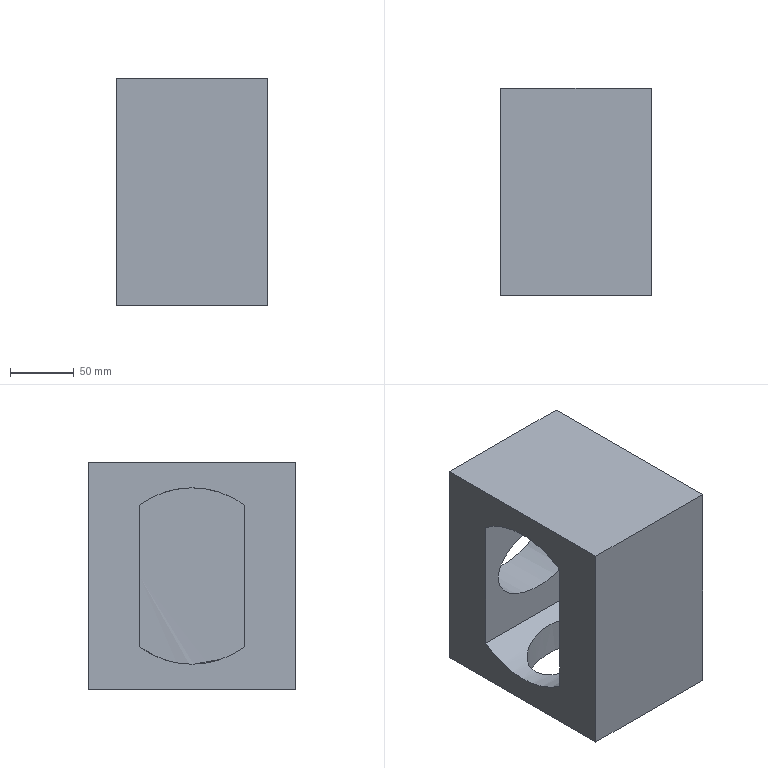Part | STEP file | 921270125 | 1 solid | 15 faces | box 118 x 162 x 178 mm | volume 2037441 mm3 | plane 9 | spline 4 | cylinder 2 | commonest cylinder face diameters 138 x2